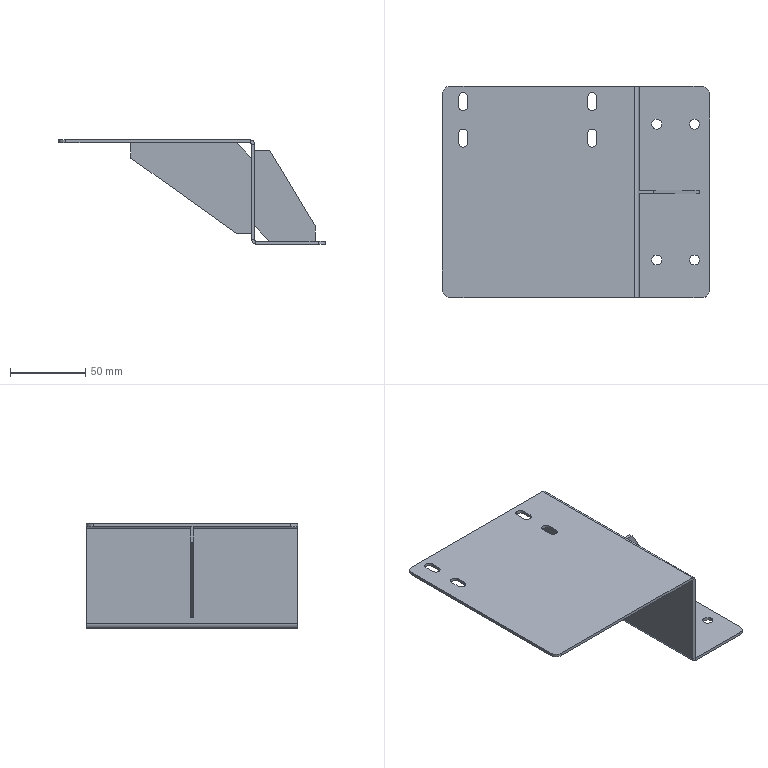Part | NX | features BREP 3 | 3 solids | 66 faces | box 177 x 140 x 69 mm | volume 76272 mm3 | plane 42 | cylinder 24 | commonest cylinder face diameters 6 x8 6.6 x8 10 x4 1.473 x2 5.473 x2